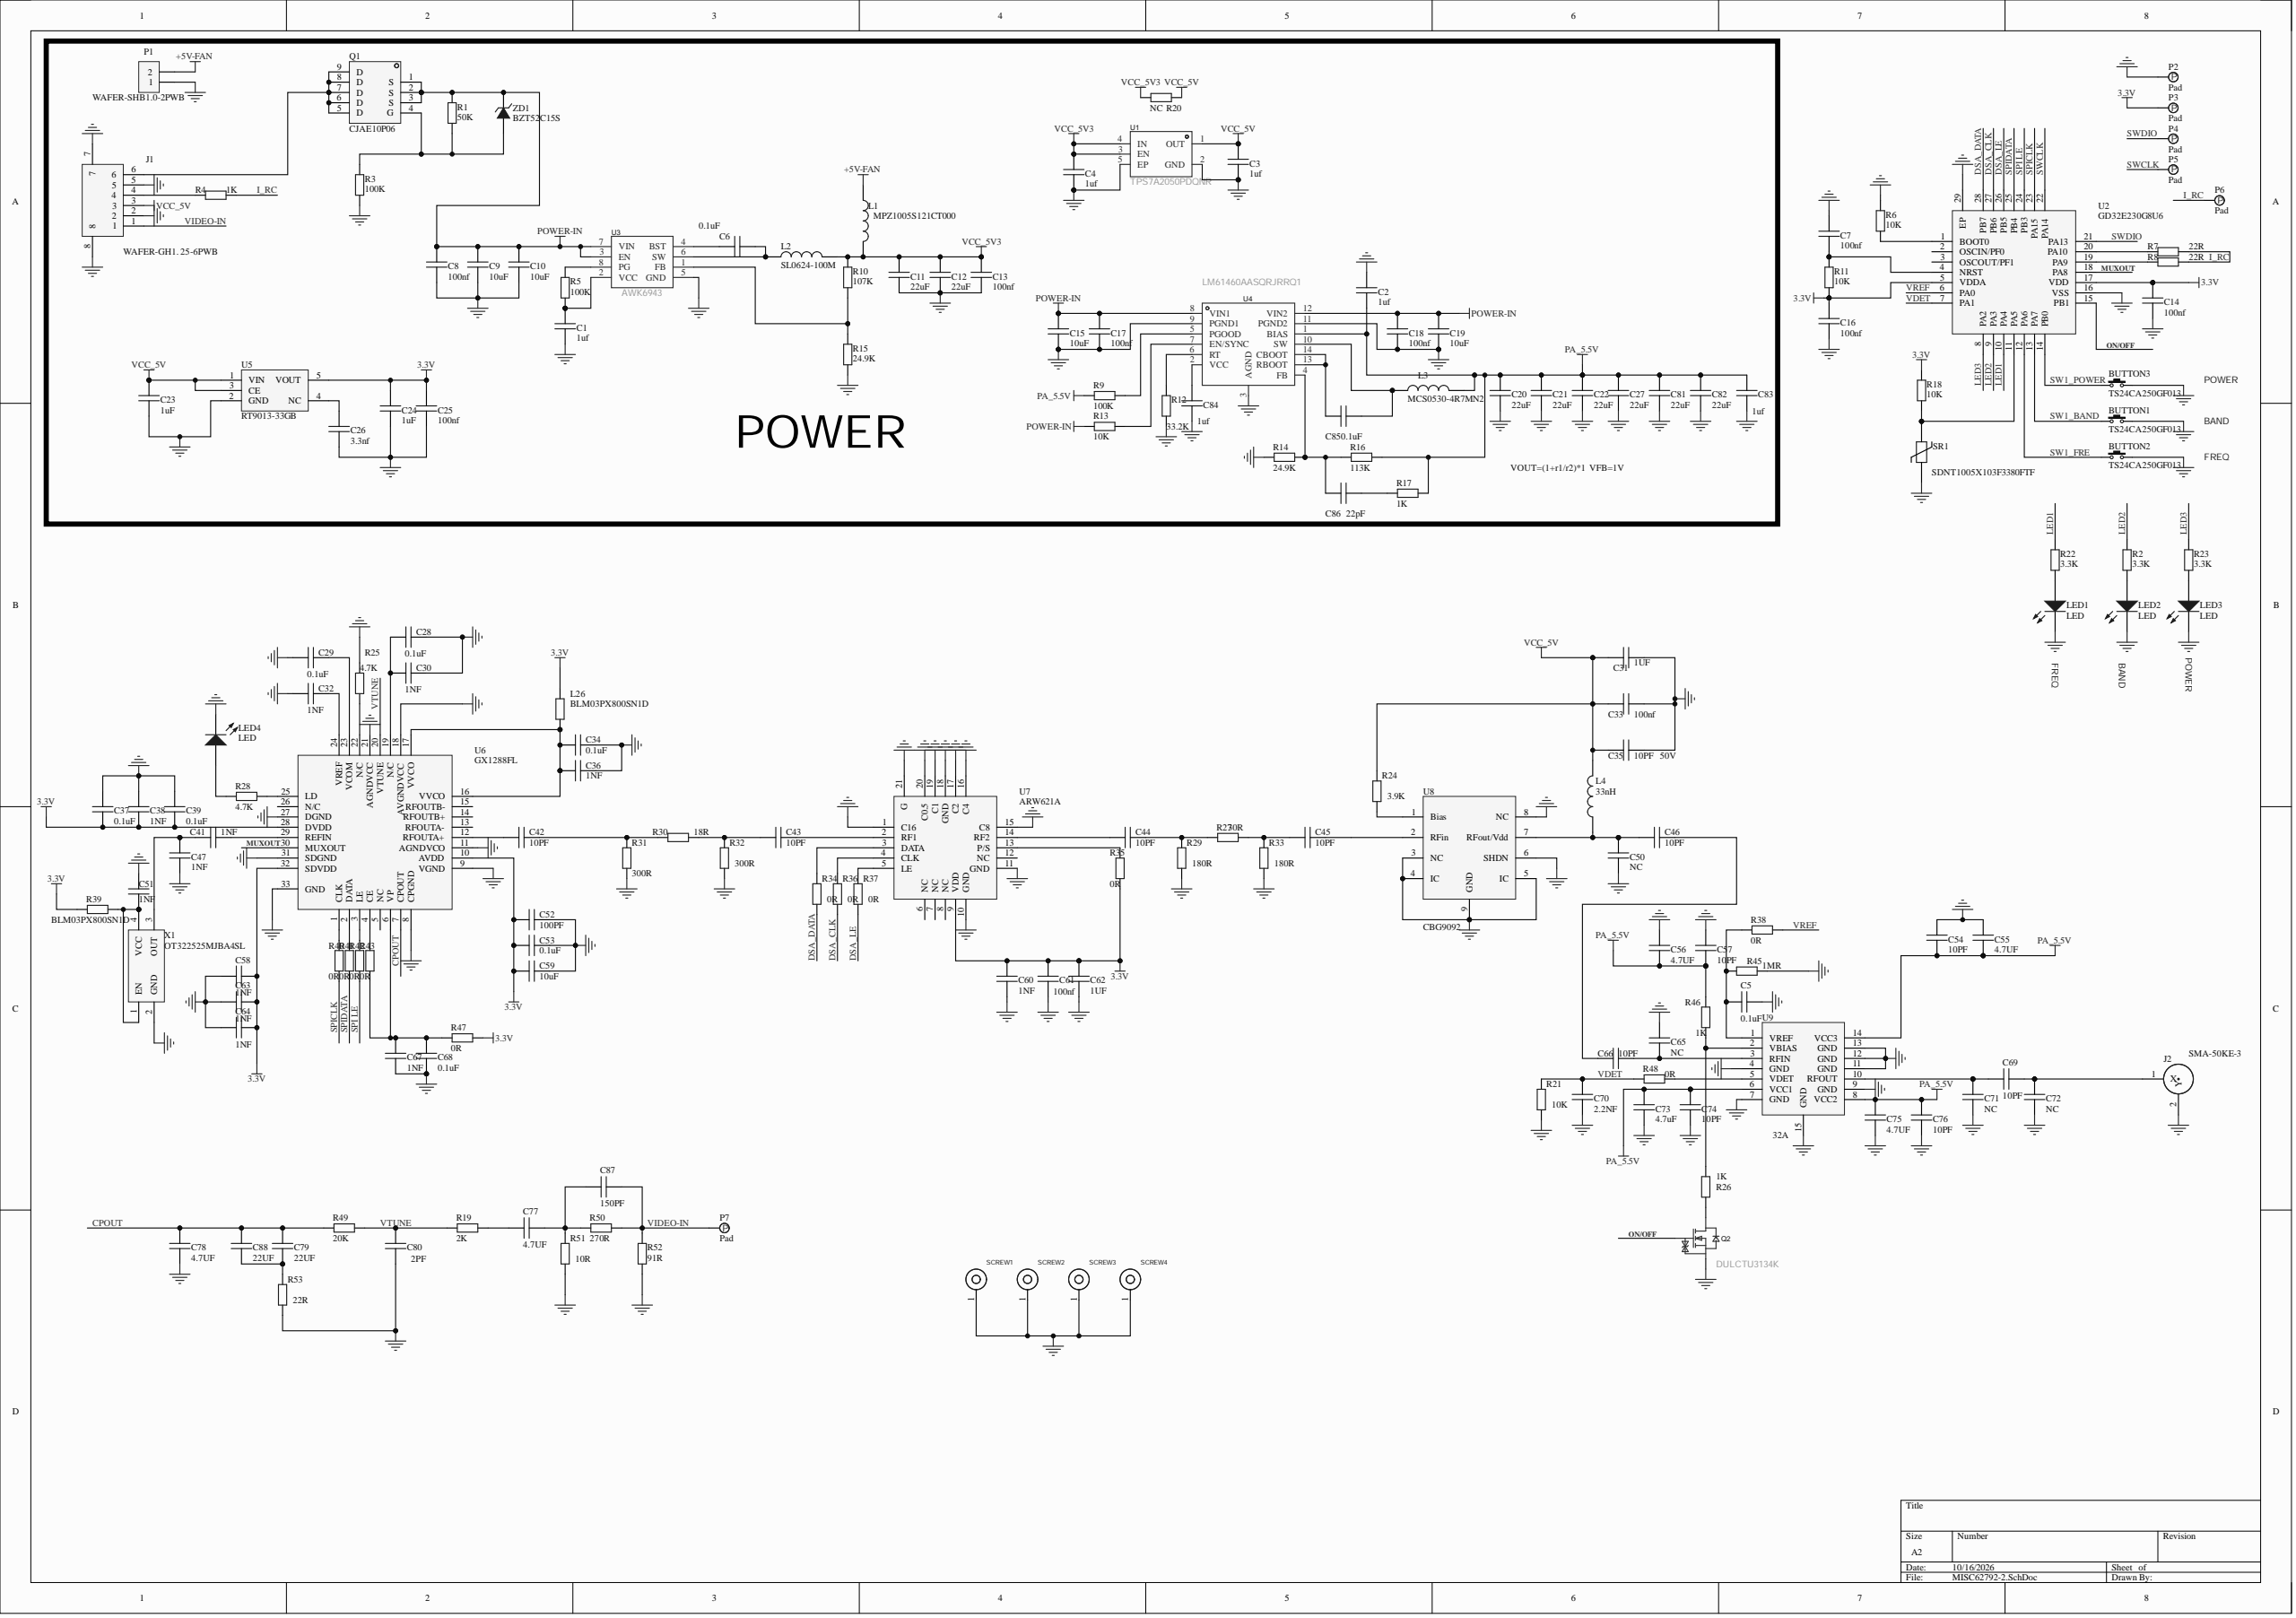Circuit board | Altium Designer | 176 parts | 94 nets
Bill of materials:
Comment,Description,Designator,Footprint,LibRef,Quantity
"TS24CA250GF013","3x6 tactile switch","BUTTON1, BUTTON2, BUTTON3","SW-SMD_L4.7-W3.5-P3.35-EH","TSW 3x6","3"
"1uf","","C1, C2, C3, C4, C83, C84","C0603","100nf","6"
"0.1uF","","C5, C6, C85","C0402","100nf","3"
"100nf","","C7, C14, C16","C0201","100nf","3"
"100nf","","C8, C13, C17, C18, C25, C33, C61","C0402","100nf","7"
"10uF","","C9, C10, C15, C19","C0805","100nf","4"
"22uF","","C11, C12, C20, C21, C22, C27, C81, C82","C0603","100nf","8"
"1uF","","C23, C24, C31, C62","C0402","100nf","4"
"3.3nf","","C26","C0402","100nf","1"
"0.1uF","","C28, C29, C34, C37, C39, C53, C68","C0201","100nf","7"
"1NF","","C30, C32, C36, C38, C41, C47, C51, C58, C63, C64, C67","C0201","100nf","11"
"10PF   50V","","C35","C0402","100nf","1"
"10PF","","C42, C43, C44, C45, C46, C54, C57, C66, C69, C74, C76","C0402","100nf","11"
"NC","","C50, C65, C71, C72","C0402","100nf","4"
"100PF","","C52","C0201","100nf","1"
"4.7UF","","C55, C56, C73, C75","C0603","100nf","4"
"10uF","","C59","C0402","100nf","1"
"1NF","","C60","C0402","100nf","1"
"2.2NF","","C70","C0402","100nf","1"
"4.7UF","","C77, C78","C0402","100nf","2"
"22UF","","C79, C88","C0402","100nf","2"
"2PF","","C80","C0402","100nf","1"
"22pF","","C86","C0402","100nf","1"
"150PF","","C87","C0402","100nf","1"
"WAFER-GH1. 25-6PWB","","J1","SMD_6P-P1.25_XUNPU_WAFER-GH1.25-6PWB","WAFER-GH1. 25-6PWB","1"
"SMA-50KE-3","","J2","SMA-FP-945G","SMA-50KE-3","1"
"MPZ1005S121CT000","Color-ring inductor","L1","L0402","L-AL","1"
"SL0624-100M","Color-ring inductor","L2","IND-SMD_L7.1-W6.6","L-AL","1"
"MCS0530-4R7MN2","Color-ring inductor","L3","IND-SMD_L5.2-W5.2_YSPI0530","L-AL","1"
"33nH","Color-ring inductor","L4","L0402","L-AL","1"
"BLM03PX800SN1D","SMD resistor","L26, R39","L0201","R","2"
"LED","LED","LED1, LED2, LED3, LED4","LED0402","LED0","4"
"WAFER-SHB1.0-2PWB","2P connector","P1","SMD_2P-WAFER-SHB1.0-2PWB","Header 2","1"
"Pad","","P2, P3, P4, P5, P6, P7","PAD","Pad","6"
"CJAE10P06","","Q1","DFN-8_L3.0-W3.0-P0.65-BL_G48N03D3","CJAE10P06","1"
"DULCTU3134K","","Q2","SOT-523-3_L1.6-W0.8-P0.50-LS1.6-BR-1","2N7002T_C5224243","1"
"50K","SMD resistor","R1","R0402","R","1"
"3.3K","SMD resistor","R2, R22, R23","R0402","R","3"
"100K","SMD resistor","R3, R5, R9","R0402","R","3"
"1K","SMD resistor","R4, R17, R26, R46","R0402","R","4"
"10K","SMD resistor","R6, R11, R18","R0201","R","3"
"22R","SMD resistor","R7, R8","R0201","R","2"
"107K","SMD resistor","R10","R0402","R","1"
"33.2K","SMD resistor","R12","R0402","R","1"
"10K","SMD resistor","R13, R21","R0402","R","2"
"24.9K","SMD resistor","R14, R15","R0402","R","2"
"113K","SMD resistor","R16","R0402","R","1"
"2K","SMD resistor","R19","R0402","R","1"
"NC","SMD resistor","R20","R0402","R","1"
"3.9K","SMD resistor","R24","R0402","R","1"
"4.7K","SMD resistor","R25, R28","R0201","R","2"
"30R","SMD resistor","R27","R0402","R","1"
"180R","SMD resistor","R29, R33","R0402","R","2"
"18R","SMD resistor","R30","R0402","R","1"
"300R","SMD resistor","R31, R32","R0402","R","2"
"0R","SMD resistor","R34, R35, R36, R37, R38, R48","R0402","R","6"
"0R","SMD resistor","R40, R41, R42, R43, R47","R0201","R","5"
"1MR","SMD resistor","R45","R0402","R","1"
"20K","SMD resistor","R49","R0402","R","1"
"270R","SMD resistor","R50","R0402","R","1"
"10R","SMD resistor","R51","R0402","R","1"
"91R","SMD resistor","R52","R0402","R","1"
"22R","SMD resistor","R53","R0402","R","1"
"MARK_4","MARK Symble","SCREW1, SCREW2, SCREW3, SCREW4","M2","MARK_4","4"
"SDNT1005X103F3380FTF","","SR1","R0402","SDNT1005X103F3380FTF","1"
"TPS7A2050PDQNR","","U1","X2SON-4_L1.0-W1.0-P0.65-TL-EP","TPS7A2050PDQNR","1"
"GD32E230G8U6","","U2","QFN-28_L4.0-W4.0-P0.40-BL-EP2.8","GD32E230G8U6","1"
"AWK6943","","U3","QFN-8_L3.0-W3.0-P0.65-BL","TPS54327DDAR","1"
"LM61460AASQRJRRQ1","","U4","VQFN-14-HR_L4.0-W3.5-TL_LM61460AASQRJRRQ1","LM61460AASQRJRRQ1","1"
"RT9013-33GB","","U5","SOT-23-5_L3.0-W1.7-P0.95-LS2.8-BL","RT9013-33GB","1"
"GX1288FL","","U6","QFN-32_L5.0-W5.0-P0.50","GX1288FL","1"
"ARW621A","","U7","QFN-20_L4.0-W4.0-P0.50-TL-EP2.2","ARW621A","1"
"CBG9092","","U8","CBG9092","CBG9092","1"
"32A","","U9","AU64XX","GCM3527(3.3G-3.8G)","1"
"OT322525MJBA4SL","4-pin active crystal oscillator","X1","SMD3225","XTAL-ACT-4P","1"
"BZT52C15S","5.1V/1W Zener diode","ZD1","SOD-323_L1.7-W1.3-LS2.6-RD","1N4733","1"
Netlist (Protel format):
[
BUTTON1
SW-SMD_L4.7-W3.5-P3.35-EH
TS24CA250GF013



]
[
BUTTON2
SW-SMD_L4.7-W3.5-P3.35-EH
TS24CA250GF013



]
[
BUTTON3
SW-SMD_L4.7-W3.5-P3.35-EH
TS24CA250GF013



]
[
C1
C0603
1uf



]
[
C2
C0603
1uf



]
[
C3
C0603
1uf



]
[
C4
C0603
1uf



]
[
C5
C0402
0.1uF



]
[
C6
C0402
0.1uF



]
[
C7
C0201
100nf



]
[
C8
C0402
100nf



]
[
C9
C0805
10uF



]
[
C10
C0805
10uF



]
[
C11
C0603
22uF



]
[
C12
C0603
22uF



]
[
C13
C0402
100nf



]
[
C14
C0201
100nf



]
[
C15
C0805
10uF



]
[
C16
C0201
100nf



]
[
C17
C0402
100nf



]
[
C18
C0402
100nf



]
[
C19
C0805
10uF



]
[
C20
C0603
22uF



]
[
C21
C0603
22uF



]
[
C22
C0603
22uF



]
[
C23
C0402
1uF



]
[
C24
C0402
1uF



]
[
C25
C0402
100nf



]
[
C26
C0402
3.3nf



]
[
C27
C0603
22uF



]
[
C28
C0201
0.1uF



]
[
C29
C0201
0.1uF



]
[
C30
C0201
1NF



]
[
C31
C0402
1UF



]
[
C32
C0201
1NF



]
[
C33
C0402
100nf



]
[
C34
C0201
0.1uF



]
[
C35
C0402
10PF   50V



]
[
C36
C0201
1NF



]
[
C37
C0201
0.1uF



]
[
C38
C0201
1NF



]
[
C39
C0201
0.1uF



]
[
C41
C0201
1NF



]
[
C42
C0402
10PF



]
[
C43
C0402
10PF



]
[
C44
C0402
10PF



]
[
C45
C0402
10PF



]
[
C46
C0402
10PF



]
[
C47
C0201
1NF



]
[
C50
C0402
NC



]
[
C51
C0201
1NF



]
[
C52
C0201
100PF



]
[
C53
C0201
0.1uF



]
[
C54
C0402
10PF



]
[
C55
C0603
4.7UF



]
[
C56
C0603
4.7UF



]
[
C57
C0402
10PF



]
[
C58
C0201
1NF



]
[
C59
C0402
10uF



]
[
C60
C0402
1NF



]
[
C61
C0402
100nf



]
[
C62
C0402
1UF



]
[
C63
C0201
1NF



]
[
C64
C0201
1NF



]
[
C65
C0402
NC



]
[
C66
C0402
10PF



]
[
C67
C0201
1NF



]
[
C68
C0201
0.1uF



]
[
C69
C0402
10PF



]
[
C70
C0402
2.2NF



]
[
C71
C0402
NC



]
[
C72
C0402
NC



]
[
C73
C0603
4.7uF



]
[
C74
C0402
10PF



]
[
C75
C0603
4.7UF



]
[
C76
C0402
10PF



]
[
C77
C0402
4.7UF



]
[
C78
C0402
4.7UF



]
[
C79
C0402
22UF



]
[
C80
C0402
2PF



]
[
C81
C0603
22uF



]
[
C82
C0603
22uF



]
[
C83
C0603
1uf



]
[
C84
C0603
1uf



]
[
C85
C0402
0.1uF



]
[
C86
C0402
22pF



]
[
C87
C0402
150PF



]
[
C88
C0402
22UF



]
[
J1
SMD_6P-P1.25_XUNPU_WAFER-GH1.25-6PWB
WAFER-GH1. 25-6PWB



]
[
J2
SMA-FP-945G
SMA-50KE-3



]
[
L1
L0402
MPZ1005S121CT000



]
[
L2
IND-SMD_L7.1-W6.6
SL0624-100M



]
[
L3
IND-SMD_L5.2-W5.2_YSPI0530
MCS0530-4R7MN2



]
[
L4
L0402
33nH



]
[
L26
L0201
BLM03PX800SN1D



]
[
LED1
LED0402
LED



]
[
LED2
LED0402
LED



]
[
LED3
LED0402
LED



]
[
LED4
LED0402
LED



]
[
P1
SMD_2P-WAFER-SHB1.0-2PWB
WAFER-SHB1.0-2PWB



]
[
P2
PAD
Pad



]
[
P3
PAD
Pad



]
[
P4
PAD
Pad



]
[
P5
PAD
Pad



]
[
P6
PAD
Pad



]
[
P7
PAD
Pad



]
[
Q1
DFN-8_L3.0-W3.0-P0.65-BL_G48N03D3
CJAE10P06



]
[
Q2
SOT-523-3_L1.6-W0.8-P0.50-LS1.6-BR-1
DULCTU3134K



]
[
R1
R0402
50K



]
[
R2
R0402
3.3K



]
[
R3
R0402
100K



]
[
R4
R0402
1K



]
[
R5
R0402
100K



]
[
R6
R0201
10K



]
[
R7
R0201
22R



]
[
R8
R0201
22R



]
[
R9
R0402
100K



]
[
R10
R0402
107K



]
[
R11
R0201
10K



]
[
R12
R0402
33.2K



]
[
R13
R0402
10K



]
[
R14
R0402
24.9K



]
[
R15
R0402
24.9K



]
[
R16
R0402
113K



]
[
R17
R0402
1K



]
[
R18
R0201
10K



]
[
R19
R0402
2K



]
[
R20
R0402
NC



]
[
R21
R0402
10K



]
[
R22
R0402
3.3K



]
[
R23
R0402
3.3K



]
[
R24
R0402
3.9K



]
[
R25
R0201
4.7K



]
[
R26
R0402
1K



]
[
R27
R0402
30R



]
[
R28
R0201
4.7K



]
[
R29
R0402
180R



]
[
R30
R0402
18R



]
[
R31
R0402
300R



]
[
R32
R0402
300R



]
[
R33
R0402
180R



]
[
R34
R0402
0R



]
[
R35
R0402
0R



]
[
R36
R0402
0R



]
[
R37
R0402
0R



]
[
R38
R0402
0R



]
[
R39
L0201
BLM03PX800SN1D



]
[
R40
R0201
0R



]
[
R41
R0201
0R



]
[
R42
R0201
0R



]
[
R43
R0201
0R



]
[
R45
R0402
1MR



]
[
R46
R0402
1K



]
[
R47
R0201
0R



]
[
R48
R0402
0R



]
[
R49
R0402
20K



]
[
R50
R0402
270R



]
[
R51
R0402
10R



]
[
R52
R0402
91R



]
[
R53
R0402
22R



]
[
SCREW1
M2
MARK_4



]
[
SCREW2
M2
MARK_4



]
[
SCREW3
M2
MARK_4



]
[
SCREW4
M2
MARK_4



]
[
SR1
R0402
SDNT1005X103F3380FTF



]
[
U1
X2SON-4_L1.0-W1.0-P0.65-TL-EP
TPS7A2050PDQNR



]
[
U2
QFN-28_L4.0-W4.0-P0.40-BL-EP2.8
GD32E230G8U6



]
[
U3
QFN-8_L3.0-W3.0-P0.65-BL
AWK6943



]
[
U4
VQFN-14-HR_L4.0-W3.5-TL_LM61460AASQRJRRQ1
LM61460AASQRJRRQ1



]
[
U5
SOT-23-5_L3.0-W1.7-P0.95-LS2.8-BL
RT9013-33GB



]
[
U6
QFN-32_L5.0-W5.0-P0.50
GX1288FL



]
[
U7
QFN-20_L4.0-W4.0-P0.50-TL-EP2.2
ARW621A



]
[
U8
CBG9092
CBG9092



]
[
U9
AU64XX
32A



]
[
X1
SMD3225
OT322525MJBA4SL



]
[
ZD1
SOD-323_L1.7-W1.3-LS2.6-RD
BZT52C15S



]
(
VTUNE
C80-2
R19-1
R49-2
U6-20
)
(
VREF
R38-1
U2-6
)
(
VIDEO-IN
C87-1
J1-1
P7-1
R50-2
R52-1
)
(
VDET
C70-2
R21-1
R48-1
U2-7
)
(
VCC_5V3
C4-1
C11-1
C12-1
C13-1
L1-2
L2-2
R10-1
R20-2
U1-3
U1-4
)
(
VCC_5V
C3-1
C23-1
C31-2
C33-2
C35-1
J1-3
L4-2
R20-1
R24-1
U1-1
U5-1
U5-3
)
(
SWDIO
P4-1
U2-21
)
(
SWCLK
P5-1
U2-22
)
(
SW1_POWER
BUTTON3-2
U2-14
)
(
SW1_FRE
BUTTON2-2
U2-12
)
(
SW1_BAND
BUTTON1-2
U2-13
)
(
SPIDATA
R41-2
U2-25
)
(
SPICLK
R40-2
U2-23
)
(
SPI LE
R42-2
U2-24
)
(
POWER-IN
C8-1
C9-1
C10-1
C15-1
C17-1
C18-1
C19-1
Q1-1
Q1-2
Q1-3
R1-2
R13-2
U3-3
U3-7
U4-8
U4-12
ZD1-2
)
(
PA_5.5V
C2-1
C20-1
C21-1
C22-1
C27-1
C54-1
C55-1
C56-2
C57-2
C73-1
C74-1
C75-1
C76-1
C81-1
C82-1
C83-1
L3-2
R9-2
R16-1
R17-1
R46-1
U4-1
U9-6
U9-8
U9-14
)
(
ON/OFF
Q2-1
U2-15
)
(
NetR48_2
R48-2
U9-5
)
(
NetR43_1
R43-1
U6-4
)
(
NetR42_1
R42-1
U6-3
)
(
NetR41_1
R41-1
U6-2
)
(
NetR40_1
R40-1
U6-1
)
(
NetR37_1
R37-1
U7-5
)
(
NetR36_1
R36-1
U7-4
)
(
NetR35_1
R35-1
U7-13
)
(
NetR34_1
R34-1
U7-3
)
(
NetR28_2
R28-2
U6-25
)
(
NetR26_1
R26-1
R46-2
U9-2
)
(
NetR25_2
R25-2
U6-22
)
(
NetR24_2
R24-2
U8-1
)
(
NetR18_2
R18-2
SR1-1
U2-11
)
(
NetR13_1
R13-1
U4-7
)
(
NetR12_1
R12-1
U4-6
)
(
NetR10_2
R10-2
R15-1
U3-1
)
(
NetR9_1
R9-1
U4-5
)
(
NetR8_1
R8-1
U2-19
)
(
NetR7_1
R7-1
U2-20
)
(
NetR6_2
R6-2
U2-1
)
(
NetR5_2
R5-2
U3-8
)
(
NetQ2_3
Q2-3
R26-2
)
(
NetQ1_4
Q1-4
R1-1
R3-2
ZD1-1
)
(
NetLED4_1
LED4-1
R28-1
)
(
NetLED3_1
LED3-1
R23-2
)
(
NetLED2_1
LED2-1
R2-2
)
(
NetLED1_1
LED1-1
R22-2
)
(
NetJ1_6
J1-6
Q1-5
Q1-6
Q1-7
Q1-8
Q1-9
)
(
NetJ1_4
J1-4
R4-1
)
(
NetC86_2
C86-2
R17-2
)
(
NetC86_1
C86-1
R14-1
R16-2
U4-4
)
(
NetC85_2
C85-2
L3-1
U4-10
)
(
NetC85_1
C85-1
U4-13
U4-14
)
(
NetC84_1
C84-1
U4-2
)
(
NetC79_1
C79-1
C88-1
R53-1
)
(
NetC77_2
C77-2
R19-2
)
(
NetC77_1
C77-1
C87-2
R50-1
R51-1
)
(
NetC69_2
C69-2
C72-2
J2-1
)
(
NetC69_1
C69-1
C71-2
U9-10
)
(
NetC67_1
C67-1
C68-2
R43-2
R47-1
U6-6
)
(
NetC65_1
C65-1
C66-1
U9-3
)
(
NetC51_2
C51-2
R39-2
X1-1
X1-4
)
(
NetC46_2
C46-2
C66-2
)
(
NetC46_1
C46-1
C50-1
L4-1
U8-7
)
(
NetC45_2
C45-2
U8-2
)
(
NetC45_1
C45-1
R27-2
R33-1
)
(
NetC44_2
C44-2
R27-1
R29-1
)
(
NetC44_1
C44-1
U7-14
)
(
NetC43_2
C43-2
U7-2
)
(
NetC43_1
C43-1
R30-2
R32-1
)
(
NetC42_2
C42-2
R30-1
R31-1
)
(
NetC42_1
C42-1
U6-12
)
(
NetC41_2
C41-2
C47-1
X1-3
)
(
NetC41_1
C41-1
U6-29
)
(
NetC34_2
C34-2
C36-1
L26-2
U6-16
U6-17
)
(
NetC32_2
C32-2
U6-24
)
(
NetC29_1
C29-1
U6-23
)
(
NetC28_2
C28-2
C30-1
U6-19
)
(
NetC26_1
C26-1
U5-4
)
(
NetC7_2
C7-2
R11-1
U2-4
)
(
NetC6_2
C6-2
L2-1
U3-6
)
(
NetC6_1
C6-1
U3-4
)
(
NetC5_2
C5-2
R38-2
R45-1
U9-1
)
(
NetC1_1
C1-1
R5-1
U3-2
)
(
MUXOUT
U2-18
U6-30
)
(
LED3
R23-1
U2-8
)
(
LED2
R2-1
U2-9
)
(
LED1
R22-1
U2-10
)
(
I_RC
P6-1
R4-2
R7-2
R8-2
)
(
GND
BUTTON1-1
BUTTON2-1
BUTTON3-1
C1-2
C2-2
C3-2
C4-2
C5-1
C7-1
C8-2
C9-2
C10-2
C11-2
C12-2
C13-2
C14-2
C15-2
C16-2
C17-2
C18-2
C19-2
C20-2
C21-2
C22-2
C23-2
C24-2
C25-2
C26-2
C27-2
C28-1
C29-2
C30-2
C31-1
C32-1
C33-1
C34-1
C35-2
C36-2
C37-1
C38-2
C39-1
C47-2
C50-2
C51-1
C52-2
C53-1
C54-2
C55-2
C56-1
C57-1
C58-1
C59-1
C60-1
C61-1
C62-1
C63-1
C64-2
C65-2
C67-2
C68-1
C70-1
C71-1
C72-1
C73-2
C74-2
C75-2
C76-2
C78-2
C80-1
C81-2
C82-2
C83-2
C84-2
J1-2
J1-5
J1-7
J1-8
J2-2
LED1-2
LED2-2
LED3-2
LED4-2
P1-1
P2-1
Q2-2
R3-1
R6-1
R12-2
R14-2
R15-2
R21-2
R25-1
R29-2
R31-2
R32-2
R33-2
R45-2
R51-2
R52-2
R53-2
SCREW1-1
SCREW2-1
SCREW3-1
SCREW4-1
SR1-2
U1-2
U1-5
U2-16
U2-29
U3-5
U4-3
U4-9
U4-11
U5-2
U6-8
U6-9
U6-11
U6-18
U6-21
U6-27
U6-31
U6-33
U7-1
U7-10
U7-11
U7-15
U7-16
U7-17
U7-18
U7-19
U7-20
U7-21
U8-3
U8-4
U8-5
U8-6
U8-8
U8-9
U9-4
U9-7
U9-9
U9-11
U9-12
U9-13
U9-15
X1-2
)
(
DSA_LE
R37-2
U2-26
)
(
DSA_DATA
R34-2
U2-28
)
(
DSA_CLK
R36-2
U2-27
)
(
CPOUT
C78-1
C79-2
C88-2
R49-1
U6-7
)
(
+5V-FAN
L1-1
P1-2
)
(
3.3V
C14-1
C16-1
C24-1
C25-1
C37-2
C38-1
C39-2
C52-1
C53-2
C58-2
C59-2
C60-2
C61-2
C62-2
C63-2
C64-1
L26-1
P3-1
R11-2
R18-1
R35-2
R39-1
R47-2
U2-5
U2-17
U5-5
U6-10
U6-28
U6-32
U7-9
)